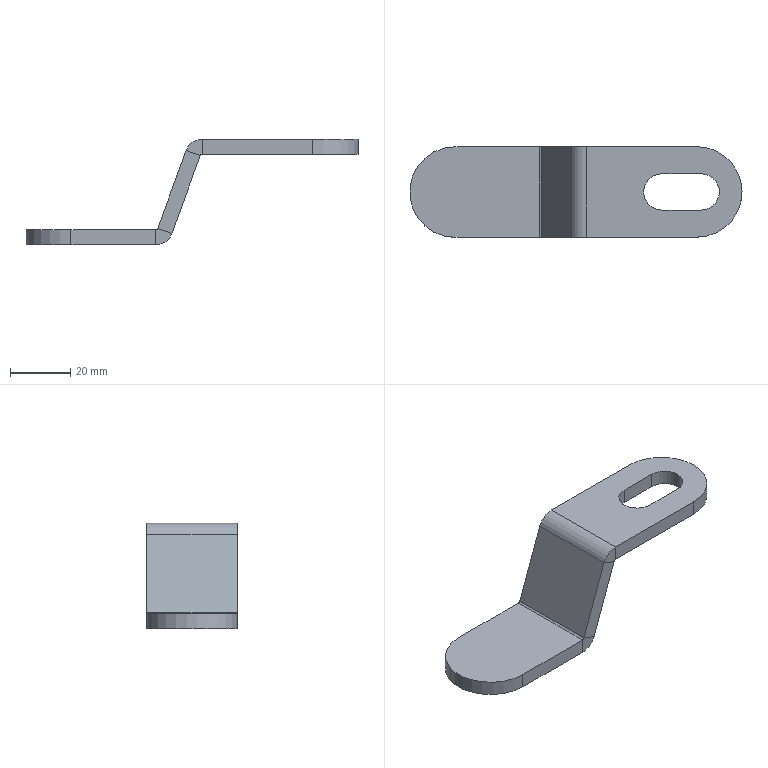Part | SolidWorks | features FlatPattern 1, Jog 1, SMBaseFlange 1, SheetMetal 1 | 1 solid | 28 faces | box 110 x 30 x 35 mm | volume 17166 mm3 | plane 18 | cylinder 10 | commonest cylinder face diameters 12 x3 30 x3 1.473 x2 11.473 x2
STEP:
#1=CARTESIAN_POINT('',(47.5,0.,25.));
#2=VERTEX_POINT('',#1);
#3=CARTESIAN_POINT('',(41.5,6.,25.));
#4=VERTEX_POINT('',#3);
#5=CARTESIAN_POINT('',(41.5,0.,25.));
#6=DIRECTION('',(0.,0.,1.));
#7=DIRECTION('',(1.,0.,0.));
#8=AXIS2_PLACEMENT_3D('',#5,#6,#7);
#9=CIRCLE('',#8,6.);
#10=EDGE_CURVE('',#2,#4,#9,.T.);
#11=ORIENTED_EDGE('',*,*,#10,.F.);
#12=CARTESIAN_POINT('',(47.5,0.,30.));
#13=VERTEX_POINT('',#12);
#14=CARTESIAN_POINT('',(47.5,0.,25.));
#15=DIRECTION('',(0.,0.,1.));
#16=VECTOR('',#15,1000.);
#17=LINE('',#14,#16);
#18=EDGE_CURVE('',#2,#13,#17,.T.);
#19=ORIENTED_EDGE('',*,*,#18,.T.);
#20=CARTESIAN_POINT('',(41.5,6.,30.));
#21=VERTEX_POINT('',#20);
#22=CARTESIAN_POINT('',(41.5,0.,30.));
#23=DIRECTION('',(0.,0.,1.));
#24=DIRECTION('',(1.,0.,0.));
#25=AXIS2_PLACEMENT_3D('',#22,#23,#24);
#26=CIRCLE('',#25,6.);
#27=EDGE_CURVE('',#13,#21,#26,.T.);
#28=ORIENTED_EDGE('',*,*,#27,.T.);
#29=CARTESIAN_POINT('',(41.5,6.,25.));
#30=DIRECTION('',(0.,0.,1.));
#31=VECTOR('',#30,1000.);
#32=LINE('',#29,#31);
#33=EDGE_CURVE('',#4,#21,#32,.T.);
#34=ORIENTED_EDGE('',*,*,#33,.F.);
#35=EDGE_LOOP('',(#11,#19,#28,#34));
#36=FACE_OUTER_BOUND('',#35,.T.);
#37=CARTESIAN_POINT('',(41.5,0.,25.));
#38=DIRECTION('',(0.,0.,1.));
#39=DIRECTION('',(1.,0.,0.));
#40=AXIS2_PLACEMENT_3D('',#37,#38,#39);
#41=CYLINDRICAL_SURFACE('',#40,6.);
#42=ADVANCED_FACE('',(#36),#41,.F.);
#43=CARTESIAN_POINT('',(40.,-15.,25.));
#44=VERTEX_POINT('',#43);
#45=CARTESIAN_POINT('',(55.,0.,25.));
#46=VERTEX_POINT('',#45);
#47=CARTESIAN_POINT('',(40.,0.,25.));
#48=DIRECTION('',(0.,0.,1.));
#49=DIRECTION('',(1.,0.,0.));
#50=AXIS2_PLACEMENT_3D('',#47,#48,#49);
#51=CIRCLE('',#50,15.);
#52=EDGE_CURVE('',#44,#46,#51,.T.);
#53=ORIENTED_EDGE('',*,*,#52,.T.);
#54=CARTESIAN_POINT('',(55.,0.,30.));
#55=VERTEX_POINT('',#54);
#56=CARTESIAN_POINT('',(55.,0.,25.));
#57=DIRECTION('',(0.,0.,1.));
#58=VECTOR('',#57,1000.);
#59=LINE('',#56,#58);
#60=EDGE_CURVE('',#46,#55,#59,.T.);
#61=ORIENTED_EDGE('',*,*,#60,.T.);
#62=CARTESIAN_POINT('',(40.,-15.,30.));
#63=VERTEX_POINT('',#62);
#64=CARTESIAN_POINT('',(40.,0.,30.));
#65=DIRECTION('',(0.,0.,1.));
#66=DIRECTION('',(1.,0.,0.));
#67=AXIS2_PLACEMENT_3D('',#64,#65,#66);
#68=CIRCLE('',#67,15.);
#69=EDGE_CURVE('',#63,#55,#68,.T.);
#70=ORIENTED_EDGE('',*,*,#69,.F.);
#71=CARTESIAN_POINT('',(40.,-15.,25.));
#72=DIRECTION('',(0.,0.,1.));
#73=VECTOR('',#72,1000.);
#74=LINE('',#71,#73);
#75=EDGE_CURVE('',#44,#63,#74,.T.);
#76=ORIENTED_EDGE('',*,*,#75,.F.);
#77=EDGE_LOOP('',(#53,#61,#70,#76));
#78=FACE_OUTER_BOUND('',#77,.T.);
#79=CARTESIAN_POINT('',(40.,0.,25.));
#80=DIRECTION('',(0.,0.,1.));
#81=DIRECTION('',(1.,0.,0.));
#82=AXIS2_PLACEMENT_3D('',#79,#80,#81);
#83=CYLINDRICAL_SURFACE('',#82,15.);
#84=ADVANCED_FACE('',(#78),#83,.T.);
#85=CARTESIAN_POINT('',(-11.285,-15.,0.4847));
#86=VERTEX_POINT('',#85);
#87=CARTESIAN_POINT('',(-1.916,-15.,26.225));
#88=VERTEX_POINT('',#87);
#89=CARTESIAN_POINT('',(-22.222,-15.,-29.564));
#90=DIRECTION('',(0.342,0.,0.9397));
#91=VECTOR('',#90,1000.);
#92=LINE('',#89,#91);
#93=EDGE_CURVE('',#86,#88,#92,.T.);
#94=ORIENTED_EDGE('',*,*,#93,.T.);
#95=CARTESIAN_POINT('',(-1.916,15.,26.225));
#96=VERTEX_POINT('',#95);
#97=CARTESIAN_POINT('',(-1.916,0.,26.225));
#98=DIRECTION('',(0.,1.,0.));
#99=VECTOR('',#98,1000.);
#100=LINE('',#97,#99);
#101=EDGE_CURVE('',#88,#96,#100,.T.);
#102=ORIENTED_EDGE('',*,*,#101,.T.);
#103=CARTESIAN_POINT('',(-11.285,15.,0.4847));
#104=VERTEX_POINT('',#103);
#105=CARTESIAN_POINT('',(-22.222,15.,-29.564));
#106=DIRECTION('',(-0.342,0.,-0.9397));
#107=VECTOR('',#106,1000.);
#108=LINE('',#105,#107);
#109=EDGE_CURVE('',#96,#104,#108,.T.);
#110=ORIENTED_EDGE('',*,*,#109,.T.);
#111=CARTESIAN_POINT('',(-11.285,0.,0.4847));
#112=DIRECTION('',(0.,1.,0.));
#113=VECTOR('',#112,1000.);
#114=LINE('',#111,#113);
#115=EDGE_CURVE('',#86,#104,#114,.T.);
#116=ORIENTED_EDGE('',*,*,#115,.F.);
#117=EDGE_LOOP('',(#94,#102,#110,#116));
#118=FACE_OUTER_BOUND('',#117,.T.);
#119=CARTESIAN_POINT('',(5.14,0.,45.611));
#120=DIRECTION('',(-0.9397,0.,0.342));
#121=DIRECTION('',(0.342,0.,0.9397));
#122=AXIS2_PLACEMENT_3D('',#119,#120,#121);
#123=PLANE('',#122);
#124=ADVANCED_FACE('',(#118),#123,.T.);
#125=ORIENTED_EDGE('',*,*,#109,.F.);
#126=CARTESIAN_POINT('',(2.782,15.,24.515));
#127=VERTEX_POINT('',#126);
#128=CARTESIAN_POINT('',(2.782,15.,24.515));
#129=DIRECTION('',(0.9397,0.,-0.342));
#130=VECTOR('',#129,1000.);
#131=LINE('',#128,#130);
#132=EDGE_CURVE('',#96,#127,#131,.T.);
#133=ORIENTED_EDGE('',*,*,#132,.T.);
#134=CARTESIAN_POINT('',(-6.586,15.,-1.225));
#135=VERTEX_POINT('',#134);
#136=CARTESIAN_POINT('',(-17.523,15.,-31.274));
#137=DIRECTION('',(-0.342,0.,-0.9397));
#138=VECTOR('',#137,1000.);
#139=LINE('',#136,#138);
#140=EDGE_CURVE('',#127,#135,#139,.T.);
#141=ORIENTED_EDGE('',*,*,#140,.T.);
#142=CARTESIAN_POINT('',(-6.586,15.,-1.225));
#143=DIRECTION('',(0.9397,0.,-0.342));
#144=VECTOR('',#143,1000.);
#145=LINE('',#142,#144);
#146=EDGE_CURVE('',#104,#135,#145,.T.);
#147=ORIENTED_EDGE('',*,*,#146,.F.);
#148=EDGE_LOOP('',(#125,#133,#141,#147));
#149=FACE_OUTER_BOUND('',#148,.T.);
#150=CARTESIAN_POINT('',(-17.523,15.,-31.274));
#151=DIRECTION('',(0.,1.,0.));
#152=DIRECTION('',(-0.9397,0.,0.342));
#153=AXIS2_PLACEMENT_3D('',#150,#151,#152);
#154=PLANE('',#153);
#155=ADVANCED_FACE('',(#149),#154,.T.);
#156=CARTESIAN_POINT('',(-6.586,-15.,-1.225));
#157=VERTEX_POINT('',#156);
#158=CARTESIAN_POINT('',(2.782,-15.,24.515));
#159=VERTEX_POINT('',#158);
#160=CARTESIAN_POINT('',(-17.523,-15.,-31.274));
#161=DIRECTION('',(0.342,0.,0.9397));
#162=VECTOR('',#161,1000.);
#163=LINE('',#160,#162);
#164=EDGE_CURVE('',#157,#159,#163,.T.);
#165=ORIENTED_EDGE('',*,*,#164,.T.);
#166=CARTESIAN_POINT('',(2.782,-15.,24.515));
#167=DIRECTION('',(-0.9397,0.,0.342));
#168=VECTOR('',#167,1000.);
#169=LINE('',#166,#168);
#170=EDGE_CURVE('',#159,#88,#169,.T.);
#171=ORIENTED_EDGE('',*,*,#170,.T.);
#172=ORIENTED_EDGE('',*,*,#93,.F.);
#173=CARTESIAN_POINT('',(-6.586,-15.,-1.225));
#174=DIRECTION('',(-0.9397,0.,0.342));
#175=VECTOR('',#174,1000.);
#176=LINE('',#173,#175);
#177=EDGE_CURVE('',#157,#86,#176,.T.);
#178=ORIENTED_EDGE('',*,*,#177,.F.);
#179=EDGE_LOOP('',(#165,#171,#172,#178));
#180=FACE_OUTER_BOUND('',#179,.T.);
#181=CARTESIAN_POINT('',(-17.523,-15.,-31.274));
#182=DIRECTION('',(0.,-1.,0.));
#183=DIRECTION('',(0.9397,0.,-0.342));
#184=AXIS2_PLACEMENT_3D('',#181,#182,#183);
#185=PLANE('',#184);
#186=ADVANCED_FACE('',(#180),#185,.T.);
#187=CARTESIAN_POINT('',(2.782,0.,24.515));
#188=DIRECTION('',(0.,1.,0.));
#189=VECTOR('',#188,1000.);
#190=LINE('',#187,#189);
#191=EDGE_CURVE('',#159,#127,#190,.T.);
#192=ORIENTED_EDGE('',*,*,#191,.F.);
#193=ORIENTED_EDGE('',*,*,#164,.F.);
#194=CARTESIAN_POINT('',(-6.586,0.,-1.225));
#195=DIRECTION('',(0.,1.,0.));
#196=VECTOR('',#195,1000.);
#197=LINE('',#194,#196);
#198=EDGE_CURVE('',#157,#135,#197,.T.);
#199=ORIENTED_EDGE('',*,*,#198,.T.);
#200=ORIENTED_EDGE('',*,*,#140,.F.);
#201=EDGE_LOOP('',(#192,#193,#199,#200));
#202=FACE_OUTER_BOUND('',#201,.T.);
#203=CARTESIAN_POINT('',(9.838,0.,43.901));
#204=DIRECTION('',(-0.9397,0.,0.342));
#205=DIRECTION('',(0.342,0.,0.9397));
#206=AXIS2_PLACEMENT_3D('',#203,#204,#205);
#207=PLANE('',#206);
#208=ADVANCED_FACE('',(#202),#207,.F.);
#209=CARTESIAN_POINT('',(-40.,15.,0.));
#210=VERTEX_POINT('',#209);
#211=CARTESIAN_POINT('',(-40.,-15.,0.));
#212=VERTEX_POINT('',#211);
#213=CARTESIAN_POINT('',(-40.,0.,0.));
#214=DIRECTION('',(0.,0.,1.));
#215=DIRECTION('',(1.,0.,0.));
#216=AXIS2_PLACEMENT_3D('',#213,#214,#215);
#217=CIRCLE('',#216,15.);
#218=EDGE_CURVE('',#210,#212,#217,.T.);
#219=ORIENTED_EDGE('',*,*,#218,.F.);
#220=CARTESIAN_POINT('',(-40.,15.,-5.));
#221=VERTEX_POINT('',#220);
#222=CARTESIAN_POINT('',(-40.,15.,-5.));
#223=DIRECTION('',(0.,0.,1.));
#224=VECTOR('',#223,1000.);
#225=LINE('',#222,#224);
#226=EDGE_CURVE('',#221,#210,#225,.T.);
#227=ORIENTED_EDGE('',*,*,#226,.F.);
#228=CARTESIAN_POINT('',(-40.,-15.,-5.));
#229=VERTEX_POINT('',#228);
#230=CARTESIAN_POINT('',(-40.,0.,-5.));
#231=DIRECTION('',(0.,0.,1.));
#232=DIRECTION('',(1.,0.,0.));
#233=AXIS2_PLACEMENT_3D('',#230,#231,#232);
#234=CIRCLE('',#233,15.);
#235=EDGE_CURVE('',#221,#229,#234,.T.);
#236=ORIENTED_EDGE('',*,*,#235,.T.);
#237=CARTESIAN_POINT('',(-40.,-15.,-5.));
#238=DIRECTION('',(0.,0.,1.));
#239=VECTOR('',#238,1000.);
#240=LINE('',#237,#239);
#241=EDGE_CURVE('',#229,#212,#240,.T.);
#242=ORIENTED_EDGE('',*,*,#241,.T.);
#243=EDGE_LOOP('',(#219,#227,#236,#242));
#244=FACE_OUTER_BOUND('',#243,.T.);
#245=CARTESIAN_POINT('',(-40.,0.,-5.));
#246=DIRECTION('',(0.,0.,1.));
#247=DIRECTION('',(1.,0.,0.));
#248=AXIS2_PLACEMENT_3D('',#245,#246,#247);
#249=CYLINDRICAL_SURFACE('',#248,15.);
#250=ADVANCED_FACE('',(#244),#249,.T.);
#251=CARTESIAN_POINT('',(-11.977,-15.,-5.));
#252=VERTEX_POINT('',#251);
#253=CARTESIAN_POINT('',(-11.977,15.,-5.));
#254=VERTEX_POINT('',#253);
#255=CARTESIAN_POINT('',(-11.977,0.,-5.));
#256=DIRECTION('',(0.,1.,0.));
#257=VECTOR('',#256,1000.);
#258=LINE('',#255,#257);
#259=EDGE_CURVE('',#252,#254,#258,.T.);
#260=ORIENTED_EDGE('',*,*,#259,.F.);
#261=CARTESIAN_POINT('',(-40.,-15.,-5.));
#262=DIRECTION('',(1.,0.,0.));
#263=VECTOR('',#262,1000.);
#264=LINE('',#261,#263);
#265=EDGE_CURVE('',#229,#252,#264,.T.);
#266=ORIENTED_EDGE('',*,*,#265,.F.);
#267=ORIENTED_EDGE('',*,*,#235,.F.);
#268=CARTESIAN_POINT('',(-40.,15.,-5.));
#269=DIRECTION('',(-1.,0.,0.));
#270=VECTOR('',#269,1000.);
#271=LINE('',#268,#270);
#272=EDGE_CURVE('',#254,#221,#271,.T.);
#273=ORIENTED_EDGE('',*,*,#272,.F.);
#274=EDGE_LOOP('',(#260,#266,#267,#273));
#275=FACE_OUTER_BOUND('',#274,.T.);
#276=CARTESIAN_POINT('',(40.,0.,-5.));
#277=DIRECTION('',(0.,0.,1.));
#278=DIRECTION('',(1.,0.,0.));
#279=AXIS2_PLACEMENT_3D('',#276,#277,#278);
#280=PLANE('',#279);
#281=ADVANCED_FACE('',(#275),#280,.F.);
#282=ORIENTED_EDGE('',*,*,#265,.T.);
#283=CARTESIAN_POINT('',(-11.977,-15.,0.));
#284=VERTEX_POINT('',#283);
#285=CARTESIAN_POINT('',(-11.977,-15.,-5.));
#286=DIRECTION('',(0.,0.,1.));
#287=VECTOR('',#286,1000.);
#288=LINE('',#285,#287);
#289=EDGE_CURVE('',#252,#284,#288,.T.);
#290=ORIENTED_EDGE('',*,*,#289,.T.);
#291=CARTESIAN_POINT('',(-40.,-15.,0.));
#292=DIRECTION('',(1.,0.,0.));
#293=VECTOR('',#292,1000.);
#294=LINE('',#291,#293);
#295=EDGE_CURVE('',#212,#284,#294,.T.);
#296=ORIENTED_EDGE('',*,*,#295,.F.);
#297=ORIENTED_EDGE('',*,*,#241,.F.);
#298=EDGE_LOOP('',(#282,#290,#296,#297));
#299=FACE_OUTER_BOUND('',#298,.T.);
#300=CARTESIAN_POINT('',(-40.,-15.,-5.));
#301=DIRECTION('',(0.,-1.,0.));
#302=DIRECTION('',(0.,0.,-1.));
#303=AXIS2_PLACEMENT_3D('',#300,#301,#302);
#304=PLANE('',#303);
#305=ADVANCED_FACE('',(#299),#304,.T.);
#306=ORIENTED_EDGE('',*,*,#295,.T.);
#307=CARTESIAN_POINT('',(-11.977,15.,0.));
#308=VERTEX_POINT('',#307);
#309=CARTESIAN_POINT('',(-11.977,0.,0.));
#310=DIRECTION('',(0.,1.,0.));
#311=VECTOR('',#310,1000.);
#312=LINE('',#309,#311);
#313=EDGE_CURVE('',#284,#308,#312,.T.);
#314=ORIENTED_EDGE('',*,*,#313,.T.);
#315=CARTESIAN_POINT('',(-40.,15.,0.));
#316=DIRECTION('',(-1.,0.,0.));
#317=VECTOR('',#316,1000.);
#318=LINE('',#315,#317);
#319=EDGE_CURVE('',#308,#210,#318,.T.);
#320=ORIENTED_EDGE('',*,*,#319,.T.);
#321=ORIENTED_EDGE('',*,*,#218,.T.);
#322=EDGE_LOOP('',(#306,#314,#320,#321));
#323=FACE_OUTER_BOUND('',#322,.T.);
#324=CARTESIAN_POINT('',(40.,0.,0.));
#325=DIRECTION('',(0.,0.,1.));
#326=DIRECTION('',(1.,0.,0.));
#327=AXIS2_PLACEMENT_3D('',#324,#325,#326);
#328=PLANE('',#327);
#329=ADVANCED_FACE('',(#323),#328,.T.);
#330=ORIENTED_EDGE('',*,*,#319,.F.);
#331=CARTESIAN_POINT('',(-11.977,15.,-5.));
#332=DIRECTION('',(0.,0.,-1.));
#333=VECTOR('',#332,1000.);
#334=LINE('',#331,#333);
#335=EDGE_CURVE('',#308,#254,#334,.T.);
#336=ORIENTED_EDGE('',*,*,#335,.T.);
#337=ORIENTED_EDGE('',*,*,#272,.T.);
#338=ORIENTED_EDGE('',*,*,#226,.T.);
#339=EDGE_LOOP('',(#330,#336,#337,#338));
#340=FACE_OUTER_BOUND('',#339,.T.);
#341=CARTESIAN_POINT('',(-40.,15.,-5.));
#342=DIRECTION('',(0.,1.,0.));
#343=DIRECTION('',(0.,0.,1.));
#344=AXIS2_PLACEMENT_3D('',#341,#342,#343);
#345=PLANE('',#344);
#346=ADVANCED_FACE('',(#340),#345,.T.);
#347=ORIENTED_EDGE('',*,*,#177,.T.);
#348=CARTESIAN_POINT('',(-11.977,-15.,0.7366));
#349=DIRECTION('',(0.,1.,0.));
#350=DIRECTION('',(1.,0.,0.));
#351=AXIS2_PLACEMENT_3D('',#348,#349,#350);
#352=CIRCLE('',#351,0.7366);
#353=EDGE_CURVE('',#86,#284,#352,.T.);
#354=ORIENTED_EDGE('',*,*,#353,.T.);
#355=ORIENTED_EDGE('',*,*,#289,.F.);
#356=CARTESIAN_POINT('',(-11.977,-15.,0.7366));
#357=DIRECTION('',(0.,1.,0.));
#358=DIRECTION('',(0.,0.,-1.));
#359=AXIS2_PLACEMENT_3D('',#356,#357,#358);
#360=CIRCLE('',#359,5.737);
#361=EDGE_CURVE('',#157,#252,#360,.T.);
#362=ORIENTED_EDGE('',*,*,#361,.F.);
#363=EDGE_LOOP('',(#347,#354,#355,#362));
#364=FACE_OUTER_BOUND('',#363,.T.);
#365=CARTESIAN_POINT('',(-11.977,-15.,0.7366));
#366=DIRECTION('',(0.,-1.,0.));
#367=DIRECTION('',(0.,0.,-1.));
#368=AXIS2_PLACEMENT_3D('',#365,#366,#367);
#369=PLANE('',#368);
#370=ADVANCED_FACE('',(#364),#369,.T.);
#371=ORIENTED_EDGE('',*,*,#335,.F.);
#372=CARTESIAN_POINT('',(-11.977,15.,0.7366));
#373=DIRECTION('',(0.,-1.,0.));
#374=DIRECTION('',(1.,0.,0.));
#375=AXIS2_PLACEMENT_3D('',#372,#373,#374);
#376=CIRCLE('',#375,0.7366);
#377=EDGE_CURVE('',#308,#104,#376,.T.);
#378=ORIENTED_EDGE('',*,*,#377,.T.);
#379=ORIENTED_EDGE('',*,*,#146,.T.);
#380=CARTESIAN_POINT('',(-11.977,15.,0.7366));
#381=DIRECTION('',(0.,-1.,0.));
#382=DIRECTION('',(0.,0.,1.));
#383=AXIS2_PLACEMENT_3D('',#380,#381,#382);
#384=CIRCLE('',#383,5.737);
#385=EDGE_CURVE('',#254,#135,#384,.T.);
#386=ORIENTED_EDGE('',*,*,#385,.F.);
#387=EDGE_LOOP('',(#371,#378,#379,#386));
#388=FACE_OUTER_BOUND('',#387,.T.);
#389=CARTESIAN_POINT('',(-11.977,15.,0.7366));
#390=DIRECTION('',(0.,1.,0.));
#391=DIRECTION('',(0.,0.,1.));
#392=AXIS2_PLACEMENT_3D('',#389,#390,#391);
#393=PLANE('',#392);
#394=ADVANCED_FACE('',(#388),#393,.T.);
#395=ORIENTED_EDGE('',*,*,#385,.T.);
#396=ORIENTED_EDGE('',*,*,#198,.F.);
#397=ORIENTED_EDGE('',*,*,#361,.T.);
#398=ORIENTED_EDGE('',*,*,#259,.T.);
#399=EDGE_LOOP('',(#395,#396,#397,#398));
#400=FACE_OUTER_BOUND('',#399,.T.);
#401=CARTESIAN_POINT('',(-11.977,30.67,0.7366));
#402=DIRECTION('',(0.,-1.,0.));
#403=DIRECTION('',(1.,0.,0.));
#404=AXIS2_PLACEMENT_3D('',#401,#402,#403);
#405=CYLINDRICAL_SURFACE('',#404,5.737);
#406=ADVANCED_FACE('',(#400),#405,.T.);
#407=ORIENTED_EDGE('',*,*,#377,.F.);
#408=ORIENTED_EDGE('',*,*,#313,.F.);
#409=ORIENTED_EDGE('',*,*,#353,.F.);
#410=ORIENTED_EDGE('',*,*,#115,.T.);
#411=EDGE_LOOP('',(#407,#408,#409,#410));
#412=FACE_OUTER_BOUND('',#411,.T.);
#413=CARTESIAN_POINT('',(-11.977,30.67,0.7366));
#414=DIRECTION('',(0.,-1.,0.));
#415=DIRECTION('',(1.,0.,0.));
#416=AXIS2_PLACEMENT_3D('',#413,#414,#415);
#417=CYLINDRICAL_SURFACE('',#416,0.7366);
#418=ADVANCED_FACE('',(#412),#417,.F.);
#419=CARTESIAN_POINT('',(3.475,-15.,25.));
#420=VERTEX_POINT('',#419);
#421=CARTESIAN_POINT('',(3.475,-15.,30.));
#422=VERTEX_POINT('',#421);
#423=CARTESIAN_POINT('',(3.475,-15.,25.));
#424=DIRECTION('',(0.,0.,1.));
#425=VECTOR('',#424,1000.);
#426=LINE('',#423,#425);
#427=EDGE_CURVE('',#420,#422,#426,.T.);
#428=ORIENTED_EDGE('',*,*,#427,.T.);
#429=CARTESIAN_POINT('',(3.475,-15.,24.263));
#430=DIRECTION('',(0.,-1.,0.));
#431=DIRECTION('',(1.,0.,0.));
#432=AXIS2_PLACEMENT_3D('',#429,#430,#431);
#433=CIRCLE('',#432,5.737);
#434=EDGE_CURVE('',#422,#88,#433,.T.);
#435=ORIENTED_EDGE('',*,*,#434,.T.);
#436=ORIENTED_EDGE('',*,*,#170,.F.);
#437=CARTESIAN_POINT('',(3.475,-15.,24.263));
#438=DIRECTION('',(0.,-1.,0.));
#439=DIRECTION('',(0.,0.,1.));
#440=AXIS2_PLACEMENT_3D('',#437,#438,#439);
#441=CIRCLE('',#440,0.7366);
#442=EDGE_CURVE('',#420,#159,#441,.T.);
#443=ORIENTED_EDGE('',*,*,#442,.F.);
#444=EDGE_LOOP('',(#428,#435,#436,#443));
#445=FACE_OUTER_BOUND('',#444,.T.);
#446=CARTESIAN_POINT('',(3.475,-15.,24.263));
#447=DIRECTION('',(0.,1.,0.));
#448=DIRECTION('',(0.,0.,1.));
#449=AXIS2_PLACEMENT_3D('',#446,#447,#448);
#450=PLANE('',#449);
#451=ADVANCED_FACE('',(#445),#450,.F.);
#452=ORIENTED_EDGE('',*,*,#132,.F.);
#453=CARTESIAN_POINT('',(3.475,15.,30.));
#454=VERTEX_POINT('',#453);
#455=CARTESIAN_POINT('',(3.475,15.,24.263));
#456=DIRECTION('',(0.,1.,0.));
#457=DIRECTION('',(1.,0.,0.));
#458=AXIS2_PLACEMENT_3D('',#455,#456,#457);
#459=CIRCLE('',#458,5.737);
#460=EDGE_CURVE('',#96,#454,#459,.T.);
#461=ORIENTED_EDGE('',*,*,#460,.T.);
#462=CARTESIAN_POINT('',(3.475,15.,25.));
#463=VERTEX_POINT('',#462);
#464=CARTESIAN_POINT('',(3.475,15.,25.));
#465=DIRECTION('',(0.,0.,-1.));
#466=VECTOR('',#465,1000.);
#467=LINE('',#464,#466);
#468=EDGE_CURVE('',#454,#463,#467,.T.);
#469=ORIENTED_EDGE('',*,*,#468,.T.);
#470=CARTESIAN_POINT('',(3.475,15.,24.263));
#471=DIRECTION('',(0.,1.,0.));
#472=DIRECTION('',(0.,0.,-1.));
#473=AXIS2_PLACEMENT_3D('',#470,#471,#472);
#474=CIRCLE('',#473,0.7366);
#475=EDGE_CURVE('',#127,#463,#474,.T.);
#476=ORIENTED_EDGE('',*,*,#475,.F.);
#477=EDGE_LOOP('',(#452,#461,#469,#476));
#478=FACE_OUTER_BOUND('',#477,.T.);
#479=CARTESIAN_POINT('',(3.475,15.,24.263));
#480=DIRECTION('',(0.,-1.,0.));
#481=DIRECTION('',(0.,0.,-1.));
#482=AXIS2_PLACEMENT_3D('',#479,#480,#481);
#483=PLANE('',#482);
#484=ADVANCED_FACE('',(#478),#483,.F.);
#485=ORIENTED_EDGE('',*,*,#475,.T.);
#486=CARTESIAN_POINT('',(3.475,0.,25.));
#487=DIRECTION('',(0.,1.,0.));
#488=VECTOR('',#487,1000.);
#489=LINE('',#486,#488);
#490=EDGE_CURVE('',#420,#463,#489,.T.);
#491=ORIENTED_EDGE('',*,*,#490,.F.);
#492=ORIENTED_EDGE('',*,*,#442,.T.);
#493=ORIENTED_EDGE('',*,*,#191,.T.);
#494=EDGE_LOOP('',(#485,#491,#492,#493));
#495=FACE_OUTER_BOUND('',#494,.T.);
#496=CARTESIAN_POINT('',(3.475,31.081,24.263));
#497=DIRECTION('',(0.,-1.,0.));
#498=DIRECTION('',(1.,0.,0.));
#499=AXIS2_PLACEMENT_3D('',#496,#497,#498);
#500=CYLINDRICAL_SURFACE('',#499,0.7366);
#501=ADVANCED_FACE('',(#495),#500,.F.);
#502=ORIENTED_EDGE('',*,*,#460,.F.);
#503=ORIENTED_EDGE('',*,*,#101,.F.);
#504=ORIENTED_EDGE('',*,*,#434,.F.);
#505=CARTESIAN_POINT('',(3.475,0.,30.));
#506=DIRECTION('',(0.,1.,0.));
#507=VECTOR('',#506,1000.);
#508=LINE('',#505,#507);
#509=EDGE_CURVE('',#422,#454,#508,.T.);
#510=ORIENTED_EDGE('',*,*,#509,.T.);
#511=EDGE_LOOP('',(#502,#503,#504,#510));
#512=FACE_OUTER_BOUND('',#511,.T.);
#513=CARTESIAN_POINT('',(3.475,31.081,24.263));
#514=DIRECTION('',(0.,-1.,0.));
#515=DIRECTION('',(1.,0.,0.));
#516=AXIS2_PLACEMENT_3D('',#513,#514,#515);
#517=CYLINDRICAL_SURFACE('',#516,5.737);
#518=ADVANCED_FACE('',(#512),#517,.T.);
#519=ORIENTED_EDGE('',*,*,#60,.F.);
#520=CARTESIAN_POINT('',(40.,15.,25.));
#521=VERTEX_POINT('',#520);
#522=CARTESIAN_POINT('',(40.,0.,25.));
#523=DIRECTION('',(0.,0.,1.));
#524=DIRECTION('',(1.,0.,0.));
#525=AXIS2_PLACEMENT_3D('',#522,#523,#524);
#526=CIRCLE('',#525,15.);
#527=EDGE_CURVE('',#46,#521,#526,.T.);
#528=ORIENTED_EDGE('',*,*,#527,.T.);
#529=CARTESIAN_POINT('',(40.,15.,30.));
#530=VERTEX_POINT('',#529);
#531=CARTESIAN_POINT('',(40.,15.,25.));
#532=DIRECTION('',(0.,0.,1.));
#533=VECTOR('',#532,1000.);
#534=LINE('',#531,#533);
#535=EDGE_CURVE('',#521,#530,#534,.T.);
#536=ORIENTED_EDGE('',*,*,#535,.T.);
#537=CARTESIAN_POINT('',(40.,0.,30.));
#538=DIRECTION('',(0.,0.,1.));
#539=DIRECTION('',(1.,0.,0.));
#540=AXIS2_PLACEMENT_3D('',#537,#538,#539);
#541=CIRCLE('',#540,15.);
#542=EDGE_CURVE('',#55,#530,#541,.T.);
#543=ORIENTED_EDGE('',*,*,#542,.F.);
#544=EDGE_LOOP('',(#519,#528,#536,#543));
#545=FACE_OUTER_BOUND('',#544,.T.);
#546=CARTESIAN_POINT('',(40.,0.,25.));
#547=DIRECTION('',(0.,0.,1.));
#548=DIRECTION('',(1.,0.,0.));
#549=AXIS2_PLACEMENT_3D('',#546,#547,#548);
#550=CYLINDRICAL_SURFACE('',#549,15.);
#551=ADVANCED_FACE('',(#545),#550,.T.);
#552=CARTESIAN_POINT('',(28.5,6.,30.));
#553=VERTEX_POINT('',#552);
#554=CARTESIAN_POINT('',(28.5,-6.,30.));
#555=VERTEX_POINT('',#554);
#556=CARTESIAN_POINT('',(28.5,0.,30.));
#557=DIRECTION('',(0.,0.,1.));
#558=DIRECTION('',(1.,0.,0.));
#559=AXIS2_PLACEMENT_3D('',#556,#557,#558);
#560=CIRCLE('',#559,6.);
#561=EDGE_CURVE('',#553,#555,#560,.T.);
#562=ORIENTED_EDGE('',*,*,#561,.T.);
#563=CARTESIAN_POINT('',(28.5,-6.,25.));
#564=VERTEX_POINT('',#563);
#565=CARTESIAN_POINT('',(28.5,-6.,25.));
#566=DIRECTION('',(0.,0.,1.));
#567=VECTOR('',#566,1000.);
#568=LINE('',#565,#567);
#569=EDGE_CURVE('',#564,#555,#568,.T.);
#570=ORIENTED_EDGE('',*,*,#569,.F.);
#571=CARTESIAN_POINT('',(28.5,6.,25.));
#572=VERTEX_POINT('',#571);
#573=CARTESIAN_POINT('',(28.5,0.,25.));
#574=DIRECTION('',(0.,0.,1.));
#575=DIRECTION('',(1.,0.,0.));
#576=AXIS2_PLACEMENT_3D('',#573,#574,#575);
#577=CIRCLE('',#576,6.);
#578=EDGE_CURVE('',#572,#564,#577,.T.);
#579=ORIENTED_EDGE('',*,*,#578,.F.);
#580=CARTESIAN_POINT('',(28.5,6.,25.));
#581=DIRECTION('',(0.,0.,1.));
#582=VECTOR('',#581,1000.);
#583=LINE('',#580,#582);
#584=EDGE_CURVE('',#572,#553,#583,.T.);
#585=ORIENTED_EDGE('',*,*,#584,.T.);
#586=EDGE_LOOP('',(#562,#570,#579,#585));
#587=FACE_OUTER_BOUND('',#586,.T.);
#588=CARTESIAN_POINT('',(28.5,0.,25.));
#589=DIRECTION('',(0.,0.,1.));
#590=DIRECTION('',(1.,0.,0.));
#591=AXIS2_PLACEMENT_3D('',#588,#589,#590);
#592=CYLINDRICAL_SURFACE('',#591,6.);
#593=ADVANCED_FACE('',(#587),#592,.F.);
#594=CARTESIAN_POINT('',(28.5,6.,30.));
#595=DIRECTION('',(-1.,0.,0.));
#596=VECTOR('',#595,1000.);
#597=LINE('',#594,#596);
#598=EDGE_CURVE('',#21,#553,#597,.T.);
#599=ORIENTED_EDGE('',*,*,#598,.T.);
#600=ORIENTED_EDGE('',*,*,#584,.F.);
#601=CARTESIAN_POINT('',(28.5,6.,25.));
#602=DIRECTION('',(-1.,0.,0.));
#603=VECTOR('',#602,1000.);
#604=LINE('',#601,#603);
#605=EDGE_CURVE('',#4,#572,#604,.T.);
#606=ORIENTED_EDGE('',*,*,#605,.F.);
#607=ORIENTED_EDGE('',*,*,#33,.T.);
#608=EDGE_LOOP('',(#599,#600,#606,#607));
#609=FACE_OUTER_BOUND('',#608,.T.);
#610=CARTESIAN_POINT('',(28.5,6.,25.));
#611=DIRECTION('',(0.,1.,0.));
#612=DIRECTION('',(0.,0.,1.));
#613=AXIS2_PLACEMENT_3D('',#610,#611,#612);
#614=PLANE('',#613);
#615=ADVANCED_FACE('',(#609),#614,.F.);
#616=ORIENTED_EDGE('',*,*,#18,.F.);
#617=CARTESIAN_POINT('',(41.5,-6.,25.));
#618=VERTEX_POINT('',#617);
#619=CARTESIAN_POINT('',(41.5,0.,25.));
#620=DIRECTION('',(0.,0.,1.));
#621=DIRECTION('',(1.,0.,0.));
#622=AXIS2_PLACEMENT_3D('',#619,#620,#621);
#623=CIRCLE('',#622,6.);
#624=EDGE_CURVE('',#618,#2,#623,.T.);
#625=ORIENTED_EDGE('',*,*,#624,.F.);
#626=CARTESIAN_POINT('',(41.5,-6.,30.));
#627=VERTEX_POINT('',#626);
#628=CARTESIAN_POINT('',(41.5,-6.,25.));
#629=DIRECTION('',(0.,0.,1.));
#630=VECTOR('',#629,1000.);
#631=LINE('',#628,#630);
#632=EDGE_CURVE('',#618,#627,#631,.T.);
#633=ORIENTED_EDGE('',*,*,#632,.T.);
#634=CARTESIAN_POINT('',(41.5,0.,30.));
#635=DIRECTION('',(0.,0.,1.));
#636=DIRECTION('',(1.,0.,0.));
#637=AXIS2_PLACEMENT_3D('',#634,#635,#636);
#638=CIRCLE('',#637,6.);
#639=EDGE_CURVE('',#627,#13,#638,.T.);
#640=ORIENTED_EDGE('',*,*,#639,.T.);
#641=EDGE_LOOP('',(#616,#625,#633,#640));
#642=FACE_OUTER_BOUND('',#641,.T.);
#643=CARTESIAN_POINT('',(41.5,0.,25.));
#644=DIRECTION('',(0.,0.,1.));
#645=DIRECTION('',(1.,0.,0.));
#646=AXIS2_PLACEMENT_3D('',#643,#644,#645);
#647=CYLINDRICAL_SURFACE('',#646,6.);
#648=ADVANCED_FACE('',(#642),#647,.F.);
#649=CARTESIAN_POINT('',(28.5,-6.,30.));
#650=DIRECTION('',(1.,0.,0.));
#651=VECTOR('',#650,1000.);
#652=LINE('',#649,#651);
#653=EDGE_CURVE('',#555,#627,#652,.T.);
#654=ORIENTED_EDGE('',*,*,#653,.T.);
#655=ORIENTED_EDGE('',*,*,#632,.F.);
#656=CARTESIAN_POINT('',(28.5,-6.,25.));
#657=DIRECTION('',(1.,0.,0.));
#658=VECTOR('',#657,1000.);
#659=LINE('',#656,#658);
#660=EDGE_CURVE('',#564,#618,#659,.T.);
#661=ORIENTED_EDGE('',*,*,#660,.F.);
#662=ORIENTED_EDGE('',*,*,#569,.T.);
#663=EDGE_LOOP('',(#654,#655,#661,#662));
#664=FACE_OUTER_BOUND('',#663,.T.);
#665=CARTESIAN_POINT('',(28.5,-6.,25.));
#666=DIRECTION('',(0.,-1.,0.));
#667=DIRECTION('',(0.,0.,-1.));
#668=AXIS2_PLACEMENT_3D('',#665,#666,#667);
#669=PLANE('',#668);
#670=ADVANCED_FACE('',(#664),#669,.F.);
#671=ORIENTED_EDGE('',*,*,#660,.T.);
#672=ORIENTED_EDGE('',*,*,#624,.T.);
#673=ORIENTED_EDGE('',*,*,#10,.T.);
#674=ORIENTED_EDGE('',*,*,#605,.T.);
#675=ORIENTED_EDGE('',*,*,#578,.T.);
#676=EDGE_LOOP('',(#671,#672,#673,#674,#675));
#677=FACE_BOUND('',#676,.T.);
#678=CARTESIAN_POINT('',(-59.85,-15.,25.));
#679=DIRECTION('',(1.,0.,0.));
#680=VECTOR('',#679,1000.);
#681=LINE('',#678,#680);
#682=EDGE_CURVE('',#420,#44,#681,.T.);
#683=ORIENTED_EDGE('',*,*,#682,.F.);
#684=ORIENTED_EDGE('',*,*,#490,.T.);
#685=CARTESIAN_POINT('',(-59.85,15.,25.));
#686=DIRECTION('',(-1.,0.,0.));
#687=VECTOR('',#686,1000.);
#688=LINE('',#685,#687);
#689=EDGE_CURVE('',#521,#463,#688,.T.);
#690=ORIENTED_EDGE('',*,*,#689,.F.);
#691=ORIENTED_EDGE('',*,*,#527,.F.);
#692=ORIENTED_EDGE('',*,*,#52,.F.);
#693=EDGE_LOOP('',(#683,#684,#690,#691,#692));
#694=FACE_OUTER_BOUND('',#693,.T.);
#695=CARTESIAN_POINT('',(20.15,0.,25.));
#696=DIRECTION('',(0.,0.,1.));
#697=DIRECTION('',(1.,0.,0.));
#698=AXIS2_PLACEMENT_3D('',#695,#696,#697);
#699=PLANE('',#698);
#700=ADVANCED_FACE('',(#677,#694),#699,.F.);
#701=ORIENTED_EDGE('',*,*,#468,.F.);
#702=CARTESIAN_POINT('',(-59.85,15.,30.));
#703=DIRECTION('',(-1.,0.,0.));
#704=VECTOR('',#703,1000.);
#705=LINE('',#702,#704);
#706=EDGE_CURVE('',#530,#454,#705,.T.);
#707=ORIENTED_EDGE('',*,*,#706,.F.);
#708=ORIENTED_EDGE('',*,*,#535,.F.);
#709=ORIENTED_EDGE('',*,*,#689,.T.);
#710=EDGE_LOOP('',(#701,#707,#708,#709));
#711=FACE_OUTER_BOUND('',#710,.T.);
#712=CARTESIAN_POINT('',(-59.85,15.,25.));
#713=DIRECTION('',(0.,1.,0.));
#714=DIRECTION('',(0.,0.,1.));
#715=AXIS2_PLACEMENT_3D('',#712,#713,#714);
#716=PLANE('',#715);
#717=ADVANCED_FACE('',(#711),#716,.T.);
#718=ORIENTED_EDGE('',*,*,#509,.F.);
#719=CARTESIAN_POINT('',(-59.85,-15.,30.));
#720=DIRECTION('',(1.,0.,0.));
#721=VECTOR('',#720,1000.);
#722=LINE('',#719,#721);
#723=EDGE_CURVE('',#422,#63,#722,.T.);
#724=ORIENTED_EDGE('',*,*,#723,.T.);
#725=ORIENTED_EDGE('',*,*,#69,.T.);
#726=ORIENTED_EDGE('',*,*,#542,.T.);
#727=ORIENTED_EDGE('',*,*,#706,.T.);
#728=EDGE_LOOP('',(#718,#724,#725,#726,#727));
#729=FACE_OUTER_BOUND('',#728,.T.);
#730=ORIENTED_EDGE('',*,*,#639,.F.);
#731=ORIENTED_EDGE('',*,*,#653,.F.);
#732=ORIENTED_EDGE('',*,*,#561,.F.);
#733=ORIENTED_EDGE('',*,*,#598,.F.);
#734=ORIENTED_EDGE('',*,*,#27,.F.);
#735=EDGE_LOOP('',(#730,#731,#732,#733,#734));
#736=FACE_BOUND('',#735,.T.);
#737=CARTESIAN_POINT('',(20.15,0.,30.));
#738=DIRECTION('',(0.,0.,1.));
#739=DIRECTION('',(1.,0.,0.));
#740=AXIS2_PLACEMENT_3D('',#737,#738,#739);
#741=PLANE('',#740);
#742=ADVANCED_FACE('',(#729,#736),#741,.T.);
#743=ORIENTED_EDGE('',*,*,#427,.F.);
#744=ORIENTED_EDGE('',*,*,#682,.T.);
#745=ORIENTED_EDGE('',*,*,#75,.T.);
#746=ORIENTED_EDGE('',*,*,#723,.F.);
#747=EDGE_LOOP('',(#743,#744,#745,#746));
#748=FACE_OUTER_BOUND('',#747,.T.);
#749=CARTESIAN_POINT('',(-59.85,-15.,25.));
#750=DIRECTION('',(0.,-1.,0.));
#751=DIRECTION('',(0.,0.,-1.));
#752=AXIS2_PLACEMENT_3D('',#749,#750,#751);
#753=PLANE('',#752);
#754=ADVANCED_FACE('',(#748),#753,.T.);
#755=CLOSED_SHELL('',(#42,#84,#124,#155,#186,#208,#250,#281,#305,#329,#346,#370,#394,#406,#418,#451,#484,#501,#518,#551,#593,#615,#648,#670,#700,#717,#742,#754));
#756=MANIFOLD_SOLID_BREP('',#755);
#757=CARTESIAN_POINT('',(0.,0.,0.));
#758=DIRECTION('',(0.,0.,1.));
#759=DIRECTION('',(1.,0.,0.));
#760=AXIS2_PLACEMENT_3D('',#757,#758,#759);
#761=(LENGTH_UNIT()NAMED_UNIT(*)SI_UNIT(.MILLI.,.METRE.));
#762=UNCERTAINTY_MEASURE_WITH_UNIT(LENGTH_MEASURE(0.00001),#761,'','');
#763=(NAMED_UNIT(*)PLANE_ANGLE_UNIT()SI_UNIT($,.RADIAN.));
#764=(NAMED_UNIT(*)SI_UNIT($,.STERADIAN.)SOLID_ANGLE_UNIT());
#765=(GEOMETRIC_REPRESENTATION_CONTEXT(3)GLOBAL_UNCERTAINTY_ASSIGNED_CONTEXT((#762))GLOBAL_UNIT_ASSIGNED_CONTEXT((#761,#763,#764))REPRESENTATION_CONTEXT('',''));
#766=ADVANCED_BREP_SHAPE_REPRESENTATION('',(#756,#760),#765);